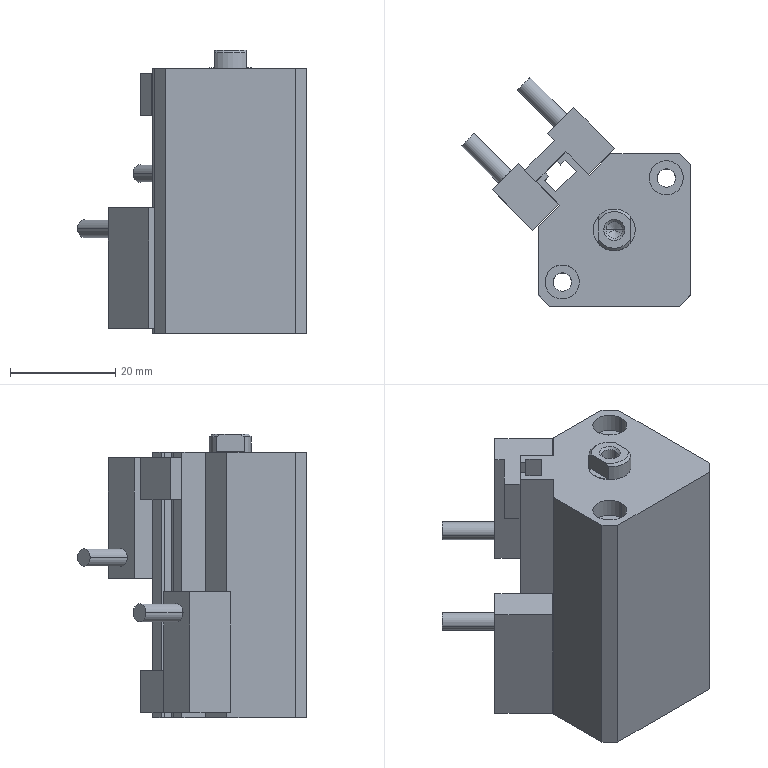Part | STEP file | CDQ2B16-20D-F7NV0 | 1 solid | 89 faces | box 43.562 x 43.562 x 54 mm | volume 41544 mm3 | plane 55 | cylinder 24 | cone 10 | commonest cylinder face diameters 6.5 x8 3.4 x4 3.5 x4 4.13 x4 3.14 x2 8 x2